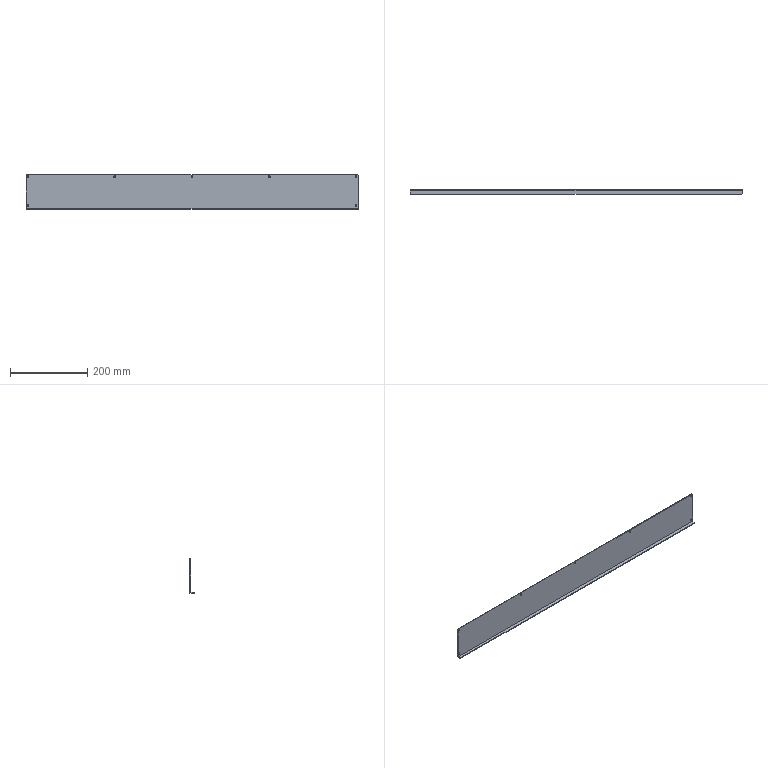Part | NX | 1 solid | 19 faces | box 860 x 10.5 x 89 mm | volume 167461 mm3 | plane 12 | cylinder 7 | commonest cylinder face diameters 4.5 x7
STEP:
#1=CARTESIAN_POINT('',(-430.,0.,-87.));
#2=VERTEX_POINT('',#1);
#3=CARTESIAN_POINT('',(-430.,-6.5,-87.));
#4=VERTEX_POINT('',#3);
#5=CARTESIAN_POINT('',(-430.,0.,-87.));
#6=DIRECTION('',(0.,-1.,0.));
#7=VECTOR('',#6,1000.);
#8=LINE('',#5,#7);
#9=EDGE_CURVE('',#2,#4,#8,.T.);
#10=ORIENTED_EDGE('',*,*,#9,.T.);
#11=CARTESIAN_POINT('',(-428.,-8.5,-87.));
#12=VERTEX_POINT('',#11);
#13=CARTESIAN_POINT('',(-430.,-6.5,-87.));
#14=DIRECTION('',(-0.7071,0.7071,0.));
#15=VECTOR('',#14,1000.);
#16=LINE('',#13,#15);
#17=EDGE_CURVE('',#4,#12,#16,.F.);
#18=ORIENTED_EDGE('',*,*,#17,.T.);
#19=CARTESIAN_POINT('',(428.,-8.5,-87.));
#20=VERTEX_POINT('',#19);
#21=CARTESIAN_POINT('',(430.,-8.5,-87.));
#22=DIRECTION('',(-1.,0.,0.));
#23=VECTOR('',#22,1000.);
#24=LINE('',#21,#23);
#25=EDGE_CURVE('',#20,#12,#24,.T.);
#26=ORIENTED_EDGE('',*,*,#25,.F.);
#27=CARTESIAN_POINT('',(430.,-6.5,-87.));
#28=VERTEX_POINT('',#27);
#29=CARTESIAN_POINT('',(428.,-8.5,-87.));
#30=DIRECTION('',(0.7071,0.7071,0.));
#31=VECTOR('',#30,1000.);
#32=LINE('',#29,#31);
#33=EDGE_CURVE('',#20,#28,#32,.T.);
#34=ORIENTED_EDGE('',*,*,#33,.T.);
#35=CARTESIAN_POINT('',(430.,0.,-87.));
#36=VERTEX_POINT('',#35);
#37=CARTESIAN_POINT('',(430.,0.,-87.));
#38=DIRECTION('',(0.,-1.,0.));
#39=VECTOR('',#38,1000.);
#40=LINE('',#37,#39);
#41=EDGE_CURVE('',#36,#28,#40,.T.);
#42=ORIENTED_EDGE('',*,*,#41,.F.);
#43=CARTESIAN_POINT('',(430.,0.,-87.));
#44=DIRECTION('',(-1.,0.,0.));
#45=VECTOR('',#44,1000.);
#46=LINE('',#43,#45);
#47=EDGE_CURVE('',#36,#2,#46,.T.);
#48=ORIENTED_EDGE('',*,*,#47,.T.);
#49=EDGE_LOOP('',(#10,#18,#26,#34,#42,#48));
#50=FACE_BOUND('',#49,.T.);
#51=CARTESIAN_POINT('',(430.,0.,-87.));
#52=DIRECTION('',(0.,0.,-1.));
#53=DIRECTION('',(-1.,0.,0.));
#54=AXIS2_PLACEMENT_3D('',#51,#52,#53);
#55=PLANE('',#54);
#56=ADVANCED_FACE('',(#50),#55,.F.);
#57=ORIENTED_EDGE('',*,*,#25,.T.);
#58=CARTESIAN_POINT('',(-428.,-8.5,-89.));
#59=VERTEX_POINT('',#58);
#60=CARTESIAN_POINT('',(-428.,-8.5,-89.));
#61=DIRECTION('',(0.,0.,-1.));
#62=VECTOR('',#61,1000.);
#63=LINE('',#60,#62);
#64=EDGE_CURVE('',#12,#59,#63,.T.);
#65=ORIENTED_EDGE('',*,*,#64,.T.);
#66=CARTESIAN_POINT('',(428.,-8.5,-89.));
#67=VERTEX_POINT('',#66);
#68=CARTESIAN_POINT('',(430.,-8.5,-89.));
#69=DIRECTION('',(-1.,0.,0.));
#70=VECTOR('',#69,1000.);
#71=LINE('',#68,#70);
#72=EDGE_CURVE('',#67,#59,#71,.T.);
#73=ORIENTED_EDGE('',*,*,#72,.F.);
#74=CARTESIAN_POINT('',(428.,-8.5,-87.));
#75=DIRECTION('',(0.,0.,1.));
#76=VECTOR('',#75,1000.);
#77=LINE('',#74,#76);
#78=EDGE_CURVE('',#67,#20,#77,.T.);
#79=ORIENTED_EDGE('',*,*,#78,.T.);
#80=EDGE_LOOP('',(#57,#65,#73,#79));
#81=FACE_BOUND('',#80,.T.);
#82=CARTESIAN_POINT('',(430.,-8.5,-89.));
#83=DIRECTION('',(0.,-1.,0.));
#84=DIRECTION('',(0.,0.,-1.));
#85=AXIS2_PLACEMENT_3D('',#82,#83,#84);
#86=PLANE('',#85);
#87=ADVANCED_FACE('',(#81),#86,.T.);
#88=ORIENTED_EDGE('',*,*,#72,.T.);
#89=CARTESIAN_POINT('',(-430.,-6.5,-89.));
#90=VERTEX_POINT('',#89);
#91=CARTESIAN_POINT('',(-3.25,-433.25,-89.));
#92=DIRECTION('',(0.7071,-0.7071,0.));
#93=VECTOR('',#92,1000.);
#94=LINE('',#91,#93);
#95=EDGE_CURVE('',#59,#90,#94,.F.);
#96=ORIENTED_EDGE('',*,*,#95,.T.);
#97=CARTESIAN_POINT('',(-430.,2.,-89.));
#98=VERTEX_POINT('',#97);
#99=CARTESIAN_POINT('',(-430.,0.,-89.));
#100=DIRECTION('',(0.,1.,0.));
#101=VECTOR('',#100,1000.);
#102=LINE('',#99,#101);
#103=EDGE_CURVE('',#98,#90,#102,.F.);
#104=ORIENTED_EDGE('',*,*,#103,.F.);
#105=CARTESIAN_POINT('',(430.,2.,-89.));
#106=VERTEX_POINT('',#105);
#107=CARTESIAN_POINT('',(430.,2.,-89.));
#108=DIRECTION('',(-1.,0.,0.));
#109=VECTOR('',#108,1000.);
#110=LINE('',#107,#109);
#111=EDGE_CURVE('',#106,#98,#110,.T.);
#112=ORIENTED_EDGE('',*,*,#111,.F.);
#113=CARTESIAN_POINT('',(430.,-6.5,-89.));
#114=VERTEX_POINT('',#113);
#115=CARTESIAN_POINT('',(430.,0.,-89.));
#116=DIRECTION('',(0.,1.,0.));
#117=VECTOR('',#116,1000.);
#118=LINE('',#115,#117);
#119=EDGE_CURVE('',#106,#114,#118,.F.);
#120=ORIENTED_EDGE('',*,*,#119,.T.);
#121=CARTESIAN_POINT('',(433.25,-3.25,-89.));
#122=DIRECTION('',(-0.7071,-0.7071,0.));
#123=VECTOR('',#122,1000.);
#124=LINE('',#121,#123);
#125=EDGE_CURVE('',#114,#67,#124,.T.);
#126=ORIENTED_EDGE('',*,*,#125,.T.);
#127=EDGE_LOOP('',(#88,#96,#104,#112,#120,#126));
#128=FACE_BOUND('',#127,.T.);
#129=CARTESIAN_POINT('',(430.,0.,-89.));
#130=DIRECTION('',(0.,0.,-1.));
#131=DIRECTION('',(-1.,0.,0.));
#132=AXIS2_PLACEMENT_3D('',#129,#130,#131);
#133=PLANE('',#132);
#134=ADVANCED_FACE('',(#128),#133,.T.);
#135=CARTESIAN_POINT('',(-425.,2.,-77.75));
#136=VERTEX_POINT('',#135);
#137=CARTESIAN_POINT('',(-425.,2.,-80.));
#138=DIRECTION('',(0.,1.,0.));
#139=DIRECTION('',(0.,0.,1.));
#140=AXIS2_PLACEMENT_3D('',#137,#138,#139);
#141=CIRCLE('',#140,2.25);
#142=EDGE_CURVE('',#136,#136,#141,.T.);
#143=ORIENTED_EDGE('',*,*,#142,.F.);
#144=EDGE_LOOP('',(#143));
#145=FACE_BOUND('',#144,.T.);
#146=CARTESIAN_POINT('',(425.,2.,-77.75));
#147=VERTEX_POINT('',#146);
#148=CARTESIAN_POINT('',(425.,2.,-80.));
#149=DIRECTION('',(0.,1.,0.));
#150=DIRECTION('',(0.,0.,1.));
#151=AXIS2_PLACEMENT_3D('',#148,#149,#150);
#152=CIRCLE('',#151,2.25);
#153=EDGE_CURVE('',#147,#147,#152,.T.);
#154=ORIENTED_EDGE('',*,*,#153,.F.);
#155=EDGE_LOOP('',(#154));
#156=FACE_BOUND('',#155,.T.);
#157=CARTESIAN_POINT('',(-425.,2.,-2.75));
#158=VERTEX_POINT('',#157);
#159=CARTESIAN_POINT('',(-425.,2.,-5.));
#160=DIRECTION('',(0.,1.,0.));
#161=DIRECTION('',(0.,0.,1.));
#162=AXIS2_PLACEMENT_3D('',#159,#160,#161);
#163=CIRCLE('',#162,2.25);
#164=EDGE_CURVE('',#158,#158,#163,.T.);
#165=ORIENTED_EDGE('',*,*,#164,.F.);
#166=EDGE_LOOP('',(#165));
#167=FACE_BOUND('',#166,.T.);
#168=CARTESIAN_POINT('',(425.,2.,-2.75));
#169=VERTEX_POINT('',#168);
#170=CARTESIAN_POINT('',(425.,2.,-5.));
#171=DIRECTION('',(0.,1.,0.));
#172=DIRECTION('',(0.,0.,1.));
#173=AXIS2_PLACEMENT_3D('',#170,#171,#172);
#174=CIRCLE('',#173,2.25);
#175=EDGE_CURVE('',#169,#169,#174,.T.);
#176=ORIENTED_EDGE('',*,*,#175,.F.);
#177=EDGE_LOOP('',(#176));
#178=FACE_BOUND('',#177,.T.);
#179=CARTESIAN_POINT('',(200.,2.,-2.75));
#180=VERTEX_POINT('',#179);
#181=CARTESIAN_POINT('',(200.,2.,-5.));
#182=DIRECTION('',(0.,1.,0.));
#183=DIRECTION('',(0.,0.,1.));
#184=AXIS2_PLACEMENT_3D('',#181,#182,#183);
#185=CIRCLE('',#184,2.25);
#186=EDGE_CURVE('',#180,#180,#185,.T.);
#187=ORIENTED_EDGE('',*,*,#186,.F.);
#188=EDGE_LOOP('',(#187));
#189=FACE_BOUND('',#188,.T.);
#190=CARTESIAN_POINT('',(-200.,2.,-2.75));
#191=VERTEX_POINT('',#190);
#192=CARTESIAN_POINT('',(-200.,2.,-5.));
#193=DIRECTION('',(0.,1.,0.));
#194=DIRECTION('',(0.,0.,1.));
#195=AXIS2_PLACEMENT_3D('',#192,#193,#194);
#196=CIRCLE('',#195,2.25);
#197=EDGE_CURVE('',#191,#191,#196,.T.);
#198=ORIENTED_EDGE('',*,*,#197,.F.);
#199=EDGE_LOOP('',(#198));
#200=FACE_BOUND('',#199,.T.);
#201=CARTESIAN_POINT('',(0.,2.,-2.75));
#202=VERTEX_POINT('',#201);
#203=CARTESIAN_POINT('',(0.,2.,-5.));
#204=DIRECTION('',(0.,1.,0.));
#205=DIRECTION('',(0.,0.,1.));
#206=AXIS2_PLACEMENT_3D('',#203,#204,#205);
#207=CIRCLE('',#206,2.25);
#208=EDGE_CURVE('',#202,#202,#207,.T.);
#209=ORIENTED_EDGE('',*,*,#208,.F.);
#210=EDGE_LOOP('',(#209));
#211=FACE_BOUND('',#210,.T.);
#212=CARTESIAN_POINT('',(428.,2.,0.));
#213=VERTEX_POINT('',#212);
#214=CARTESIAN_POINT('',(-428.,2.,0.));
#215=VERTEX_POINT('',#214);
#216=CARTESIAN_POINT('',(430.,2.,0.));
#217=DIRECTION('',(-1.,0.,0.));
#218=VECTOR('',#217,1000.);
#219=LINE('',#216,#218);
#220=EDGE_CURVE('',#213,#215,#219,.T.);
#221=ORIENTED_EDGE('',*,*,#220,.F.);
#222=CARTESIAN_POINT('',(430.,2.,-2.));
#223=VERTEX_POINT('',#222);
#224=CARTESIAN_POINT('',(429.,2.,-1.));
#225=DIRECTION('',(0.7071,0.,-0.7071));
#226=VECTOR('',#225,1000.);
#227=LINE('',#224,#226);
#228=EDGE_CURVE('',#213,#223,#227,.T.);
#229=ORIENTED_EDGE('',*,*,#228,.T.);
#230=CARTESIAN_POINT('',(430.,2.,0.));
#231=DIRECTION('',(0.,0.,-1.));
#232=VECTOR('',#231,1000.);
#233=LINE('',#230,#232);
#234=EDGE_CURVE('',#223,#106,#233,.T.);
#235=ORIENTED_EDGE('',*,*,#234,.T.);
#236=ORIENTED_EDGE('',*,*,#111,.T.);
#237=CARTESIAN_POINT('',(-430.,2.,-2.));
#238=VERTEX_POINT('',#237);
#239=CARTESIAN_POINT('',(-430.,2.,0.));
#240=DIRECTION('',(0.,0.,-1.));
#241=VECTOR('',#240,1000.);
#242=LINE('',#239,#241);
#243=EDGE_CURVE('',#238,#98,#242,.T.);
#244=ORIENTED_EDGE('',*,*,#243,.F.);
#245=CARTESIAN_POINT('',(1.,2.,429.));
#246=DIRECTION('',(-0.7071,0.,-0.7071));
#247=VECTOR('',#246,1000.);
#248=LINE('',#245,#247);
#249=EDGE_CURVE('',#238,#215,#248,.F.);
#250=ORIENTED_EDGE('',*,*,#249,.T.);
#251=EDGE_LOOP('',(#221,#229,#235,#236,#244,#250));
#252=FACE_BOUND('',#251,.T.);
#253=CARTESIAN_POINT('',(430.,2.,0.));
#254=DIRECTION('',(0.,1.,0.));
#255=DIRECTION('',(0.,0.,1.));
#256=AXIS2_PLACEMENT_3D('',#253,#254,#255);
#257=PLANE('',#256);
#258=ADVANCED_FACE('',(#145,#156,#167,#178,#189,#200,#211,#252),#257,.T.);
#259=CARTESIAN_POINT('',(428.,0.,0.));
#260=VERTEX_POINT('',#259);
#261=CARTESIAN_POINT('',(-428.,0.,0.));
#262=VERTEX_POINT('',#261);
#263=CARTESIAN_POINT('',(430.,0.,0.));
#264=DIRECTION('',(-1.,0.,0.));
#265=VECTOR('',#264,1000.);
#266=LINE('',#263,#265);
#267=EDGE_CURVE('',#260,#262,#266,.T.);
#268=ORIENTED_EDGE('',*,*,#267,.F.);
#269=CARTESIAN_POINT('',(428.,2.,0.));
#270=DIRECTION('',(0.,1.,0.));
#271=VECTOR('',#270,1000.);
#272=LINE('',#269,#271);
#273=EDGE_CURVE('',#260,#213,#272,.T.);
#274=ORIENTED_EDGE('',*,*,#273,.T.);
#275=ORIENTED_EDGE('',*,*,#220,.T.);
#276=CARTESIAN_POINT('',(-428.,0.,0.));
#277=DIRECTION('',(0.,-1.,0.));
#278=VECTOR('',#277,1000.);
#279=LINE('',#276,#278);
#280=EDGE_CURVE('',#215,#262,#279,.T.);
#281=ORIENTED_EDGE('',*,*,#280,.T.);
#282=EDGE_LOOP('',(#268,#274,#275,#281));
#283=FACE_BOUND('',#282,.T.);
#284=CARTESIAN_POINT('',(430.,0.,0.));
#285=DIRECTION('',(0.,0.,1.));
#286=DIRECTION('',(1.,0.,0.));
#287=AXIS2_PLACEMENT_3D('',#284,#285,#286);
#288=PLANE('',#287);
#289=ADVANCED_FACE('',(#283),#288,.T.);
#290=CARTESIAN_POINT('',(-425.,0.,-77.75));
#291=VERTEX_POINT('',#290);
#292=CARTESIAN_POINT('',(-425.,0.,-80.));
#293=DIRECTION('',(0.,1.,0.));
#294=DIRECTION('',(0.,0.,1.));
#295=AXIS2_PLACEMENT_3D('',#292,#293,#294);
#296=CIRCLE('',#295,2.25);
#297=EDGE_CURVE('',#291,#291,#296,.T.);
#298=ORIENTED_EDGE('',*,*,#297,.T.);
#299=EDGE_LOOP('',(#298));
#300=FACE_BOUND('',#299,.T.);
#301=CARTESIAN_POINT('',(425.,0.,-77.75));
#302=VERTEX_POINT('',#301);
#303=CARTESIAN_POINT('',(425.,0.,-80.));
#304=DIRECTION('',(0.,1.,0.));
#305=DIRECTION('',(0.,0.,1.));
#306=AXIS2_PLACEMENT_3D('',#303,#304,#305);
#307=CIRCLE('',#306,2.25);
#308=EDGE_CURVE('',#302,#302,#307,.T.);
#309=ORIENTED_EDGE('',*,*,#308,.T.);
#310=EDGE_LOOP('',(#309));
#311=FACE_BOUND('',#310,.T.);
#312=CARTESIAN_POINT('',(-425.,0.,-2.75));
#313=VERTEX_POINT('',#312);
#314=CARTESIAN_POINT('',(-425.,0.,-5.));
#315=DIRECTION('',(0.,1.,0.));
#316=DIRECTION('',(0.,0.,1.));
#317=AXIS2_PLACEMENT_3D('',#314,#315,#316);
#318=CIRCLE('',#317,2.25);
#319=EDGE_CURVE('',#313,#313,#318,.T.);
#320=ORIENTED_EDGE('',*,*,#319,.T.);
#321=EDGE_LOOP('',(#320));
#322=FACE_BOUND('',#321,.T.);
#323=CARTESIAN_POINT('',(425.,0.,-2.75));
#324=VERTEX_POINT('',#323);
#325=CARTESIAN_POINT('',(425.,0.,-5.));
#326=DIRECTION('',(0.,1.,0.));
#327=DIRECTION('',(0.,0.,1.));
#328=AXIS2_PLACEMENT_3D('',#325,#326,#327);
#329=CIRCLE('',#328,2.25);
#330=EDGE_CURVE('',#324,#324,#329,.T.);
#331=ORIENTED_EDGE('',*,*,#330,.T.);
#332=EDGE_LOOP('',(#331));
#333=FACE_BOUND('',#332,.T.);
#334=CARTESIAN_POINT('',(200.,0.,-2.75));
#335=VERTEX_POINT('',#334);
#336=CARTESIAN_POINT('',(200.,0.,-5.));
#337=DIRECTION('',(0.,1.,0.));
#338=DIRECTION('',(0.,0.,1.));
#339=AXIS2_PLACEMENT_3D('',#336,#337,#338);
#340=CIRCLE('',#339,2.25);
#341=EDGE_CURVE('',#335,#335,#340,.T.);
#342=ORIENTED_EDGE('',*,*,#341,.T.);
#343=EDGE_LOOP('',(#342));
#344=FACE_BOUND('',#343,.T.);
#345=CARTESIAN_POINT('',(-200.,0.,-2.75));
#346=VERTEX_POINT('',#345);
#347=CARTESIAN_POINT('',(-200.,0.,-5.));
#348=DIRECTION('',(0.,1.,0.));
#349=DIRECTION('',(0.,0.,1.));
#350=AXIS2_PLACEMENT_3D('',#347,#348,#349);
#351=CIRCLE('',#350,2.25);
#352=EDGE_CURVE('',#346,#346,#351,.T.);
#353=ORIENTED_EDGE('',*,*,#352,.T.);
#354=EDGE_LOOP('',(#353));
#355=FACE_BOUND('',#354,.T.);
#356=CARTESIAN_POINT('',(0.,0.,-2.75));
#357=VERTEX_POINT('',#356);
#358=CARTESIAN_POINT('',(0.,0.,-5.));
#359=DIRECTION('',(0.,1.,0.));
#360=DIRECTION('',(0.,0.,1.));
#361=AXIS2_PLACEMENT_3D('',#358,#359,#360);
#362=CIRCLE('',#361,2.25);
#363=EDGE_CURVE('',#357,#357,#362,.T.);
#364=ORIENTED_EDGE('',*,*,#363,.T.);
#365=EDGE_LOOP('',(#364));
#366=FACE_BOUND('',#365,.T.);
#367=CARTESIAN_POINT('',(430.,0.,-2.));
#368=VERTEX_POINT('',#367);
#369=CARTESIAN_POINT('',(430.,0.,0.));
#370=DIRECTION('',(0.,0.,-1.));
#371=VECTOR('',#370,1000.);
#372=LINE('',#369,#371);
#373=EDGE_CURVE('',#368,#36,#372,.T.);
#374=ORIENTED_EDGE('',*,*,#373,.F.);
#375=CARTESIAN_POINT('',(428.,0.,0.));
#376=DIRECTION('',(-0.7071,0.,0.7071));
#377=VECTOR('',#376,1000.);
#378=LINE('',#375,#377);
#379=EDGE_CURVE('',#368,#260,#378,.T.);
#380=ORIENTED_EDGE('',*,*,#379,.T.);
#381=ORIENTED_EDGE('',*,*,#267,.T.);
#382=CARTESIAN_POINT('',(-430.,0.,-2.));
#383=VERTEX_POINT('',#382);
#384=CARTESIAN_POINT('',(-430.,0.,-2.));
#385=DIRECTION('',(0.7071,0.,0.7071));
#386=VECTOR('',#385,1000.);
#387=LINE('',#384,#386);
#388=EDGE_CURVE('',#262,#383,#387,.F.);
#389=ORIENTED_EDGE('',*,*,#388,.T.);
#390=CARTESIAN_POINT('',(-430.,0.,0.));
#391=DIRECTION('',(0.,0.,-1.));
#392=VECTOR('',#391,1000.);
#393=LINE('',#390,#392);
#394=EDGE_CURVE('',#383,#2,#393,.T.);
#395=ORIENTED_EDGE('',*,*,#394,.T.);
#396=ORIENTED_EDGE('',*,*,#47,.F.);
#397=EDGE_LOOP('',(#374,#380,#381,#389,#395,#396));
#398=FACE_BOUND('',#397,.T.);
#399=CARTESIAN_POINT('',(430.,0.,0.));
#400=DIRECTION('',(0.,1.,0.));
#401=DIRECTION('',(0.,0.,1.));
#402=AXIS2_PLACEMENT_3D('',#399,#400,#401);
#403=PLANE('',#402);
#404=ADVANCED_FACE('',(#300,#311,#322,#333,#344,#355,#366,#398),#403,.F.);
#405=ORIENTED_EDGE('',*,*,#234,.F.);
#406=CARTESIAN_POINT('',(430.,0.,-2.));
#407=DIRECTION('',(0.,-1.,0.));
#408=VECTOR('',#407,1000.);
#409=LINE('',#406,#408);
#410=EDGE_CURVE('',#223,#368,#409,.T.);
#411=ORIENTED_EDGE('',*,*,#410,.T.);
#412=ORIENTED_EDGE('',*,*,#373,.T.);
#413=ORIENTED_EDGE('',*,*,#41,.T.);
#414=CARTESIAN_POINT('',(430.,-6.5,-89.));
#415=DIRECTION('',(0.,0.,-1.));
#416=VECTOR('',#415,1000.);
#417=LINE('',#414,#416);
#418=EDGE_CURVE('',#28,#114,#417,.T.);
#419=ORIENTED_EDGE('',*,*,#418,.T.);
#420=ORIENTED_EDGE('',*,*,#119,.F.);
#421=EDGE_LOOP('',(#405,#411,#412,#413,#419,#420));
#422=FACE_BOUND('',#421,.T.);
#423=CARTESIAN_POINT('',(430.,0.,0.));
#424=DIRECTION('',(-1.,0.,0.));
#425=DIRECTION('',(0.,0.,1.));
#426=AXIS2_PLACEMENT_3D('',#423,#424,#425);
#427=PLANE('',#426);
#428=ADVANCED_FACE('',(#422),#427,.F.);
#429=ORIENTED_EDGE('',*,*,#394,.F.);
#430=CARTESIAN_POINT('',(-430.,0.,-2.));
#431=DIRECTION('',(0.,1.,0.));
#432=VECTOR('',#431,1000.);
#433=LINE('',#430,#432);
#434=EDGE_CURVE('',#383,#238,#433,.T.);
#435=ORIENTED_EDGE('',*,*,#434,.T.);
#436=ORIENTED_EDGE('',*,*,#243,.T.);
#437=ORIENTED_EDGE('',*,*,#103,.T.);
#438=CARTESIAN_POINT('',(-430.,-6.5,0.));
#439=DIRECTION('',(0.,0.,1.));
#440=VECTOR('',#439,1000.);
#441=LINE('',#438,#440);
#442=EDGE_CURVE('',#90,#4,#441,.T.);
#443=ORIENTED_EDGE('',*,*,#442,.T.);
#444=ORIENTED_EDGE('',*,*,#9,.F.);
#445=EDGE_LOOP('',(#429,#435,#436,#437,#443,#444));
#446=FACE_BOUND('',#445,.T.);
#447=CARTESIAN_POINT('',(-430.,0.,0.));
#448=DIRECTION('',(-1.,0.,0.));
#449=DIRECTION('',(0.,0.,1.));
#450=AXIS2_PLACEMENT_3D('',#447,#448,#449);
#451=PLANE('',#450);
#452=ADVANCED_FACE('',(#446),#451,.T.);
#453=ORIENTED_EDGE('',*,*,#379,.F.);
#454=ORIENTED_EDGE('',*,*,#410,.F.);
#455=ORIENTED_EDGE('',*,*,#228,.F.);
#456=ORIENTED_EDGE('',*,*,#273,.F.);
#457=EDGE_LOOP('',(#453,#454,#455,#456));
#458=FACE_BOUND('',#457,.T.);
#459=CARTESIAN_POINT('',(428.,0.,0.));
#460=DIRECTION('',(0.7071,0.,0.7071));
#461=DIRECTION('',(0.,-1.,0.));
#462=AXIS2_PLACEMENT_3D('',#459,#460,#461);
#463=PLANE('',#462);
#464=ADVANCED_FACE('',(#458),#463,.T.);
#465=ORIENTED_EDGE('',*,*,#388,.F.);
#466=ORIENTED_EDGE('',*,*,#280,.F.);
#467=ORIENTED_EDGE('',*,*,#249,.F.);
#468=ORIENTED_EDGE('',*,*,#434,.F.);
#469=EDGE_LOOP('',(#465,#466,#467,#468));
#470=FACE_BOUND('',#469,.T.);
#471=CARTESIAN_POINT('',(-430.,0.,-2.));
#472=DIRECTION('',(0.7071,0.,-0.7071));
#473=DIRECTION('',(0.,1.,0.));
#474=AXIS2_PLACEMENT_3D('',#471,#472,#473);
#475=PLANE('',#474);
#476=ADVANCED_FACE('',(#470),#475,.F.);
#477=ORIENTED_EDGE('',*,*,#95,.F.);
#478=ORIENTED_EDGE('',*,*,#64,.F.);
#479=ORIENTED_EDGE('',*,*,#17,.F.);
#480=ORIENTED_EDGE('',*,*,#442,.F.);
#481=EDGE_LOOP('',(#477,#478,#479,#480));
#482=FACE_BOUND('',#481,.T.);
#483=CARTESIAN_POINT('',(-430.,-6.5,0.));
#484=DIRECTION('',(0.7071,0.7071,0.));
#485=DIRECTION('',(0.,0.,1.));
#486=AXIS2_PLACEMENT_3D('',#483,#484,#485);
#487=PLANE('',#486);
#488=ADVANCED_FACE('',(#482),#487,.F.);
#489=ORIENTED_EDGE('',*,*,#125,.F.);
#490=ORIENTED_EDGE('',*,*,#418,.F.);
#491=ORIENTED_EDGE('',*,*,#33,.F.);
#492=ORIENTED_EDGE('',*,*,#78,.F.);
#493=EDGE_LOOP('',(#489,#490,#491,#492));
#494=FACE_BOUND('',#493,.T.);
#495=CARTESIAN_POINT('',(428.,-8.5,-89.));
#496=DIRECTION('',(0.7071,-0.7071,0.));
#497=DIRECTION('',(0.,0.,-1.));
#498=AXIS2_PLACEMENT_3D('',#495,#496,#497);
#499=PLANE('',#498);
#500=ADVANCED_FACE('',(#494),#499,.T.);
#501=ORIENTED_EDGE('',*,*,#208,.T.);
#502=EDGE_LOOP('',(#501));
#503=FACE_BOUND('',#502,.T.);
#504=ORIENTED_EDGE('',*,*,#363,.F.);
#505=EDGE_LOOP('',(#504));
#506=FACE_BOUND('',#505,.T.);
#507=CARTESIAN_POINT('',(0.,2.,-5.));
#508=DIRECTION('',(0.,1.,0.));
#509=DIRECTION('',(0.,0.,1.));
#510=AXIS2_PLACEMENT_3D('',#507,#508,#509);
#511=CYLINDRICAL_SURFACE('',#510,2.25);
#512=ADVANCED_FACE('',(#503,#506),#511,.F.);
#513=ORIENTED_EDGE('',*,*,#197,.T.);
#514=EDGE_LOOP('',(#513));
#515=FACE_BOUND('',#514,.T.);
#516=ORIENTED_EDGE('',*,*,#352,.F.);
#517=EDGE_LOOP('',(#516));
#518=FACE_BOUND('',#517,.T.);
#519=CARTESIAN_POINT('',(-200.,2.,-5.));
#520=DIRECTION('',(0.,1.,0.));
#521=DIRECTION('',(0.,0.,1.));
#522=AXIS2_PLACEMENT_3D('',#519,#520,#521);
#523=CYLINDRICAL_SURFACE('',#522,2.25);
#524=ADVANCED_FACE('',(#515,#518),#523,.F.);
#525=ORIENTED_EDGE('',*,*,#186,.T.);
#526=EDGE_LOOP('',(#525));
#527=FACE_BOUND('',#526,.T.);
#528=ORIENTED_EDGE('',*,*,#341,.F.);
#529=EDGE_LOOP('',(#528));
#530=FACE_BOUND('',#529,.T.);
#531=CARTESIAN_POINT('',(200.,2.,-5.));
#532=DIRECTION('',(0.,1.,0.));
#533=DIRECTION('',(0.,0.,1.));
#534=AXIS2_PLACEMENT_3D('',#531,#532,#533);
#535=CYLINDRICAL_SURFACE('',#534,2.25);
#536=ADVANCED_FACE('',(#527,#530),#535,.F.);
#537=ORIENTED_EDGE('',*,*,#175,.T.);
#538=EDGE_LOOP('',(#537));
#539=FACE_BOUND('',#538,.T.);
#540=ORIENTED_EDGE('',*,*,#330,.F.);
#541=EDGE_LOOP('',(#540));
#542=FACE_BOUND('',#541,.T.);
#543=CARTESIAN_POINT('',(425.,2.,-5.));
#544=DIRECTION('',(0.,1.,0.));
#545=DIRECTION('',(0.,0.,1.));
#546=AXIS2_PLACEMENT_3D('',#543,#544,#545);
#547=CYLINDRICAL_SURFACE('',#546,2.25);
#548=ADVANCED_FACE('',(#539,#542),#547,.F.);
#549=ORIENTED_EDGE('',*,*,#164,.T.);
#550=EDGE_LOOP('',(#549));
#551=FACE_BOUND('',#550,.T.);
#552=ORIENTED_EDGE('',*,*,#319,.F.);
#553=EDGE_LOOP('',(#552));
#554=FACE_BOUND('',#553,.T.);
#555=CARTESIAN_POINT('',(-425.,2.,-5.));
#556=DIRECTION('',(0.,1.,0.));
#557=DIRECTION('',(0.,0.,1.));
#558=AXIS2_PLACEMENT_3D('',#555,#556,#557);
#559=CYLINDRICAL_SURFACE('',#558,2.25);
#560=ADVANCED_FACE('',(#551,#554),#559,.F.);
#561=ORIENTED_EDGE('',*,*,#153,.T.);
#562=EDGE_LOOP('',(#561));
#563=FACE_BOUND('',#562,.T.);
#564=ORIENTED_EDGE('',*,*,#308,.F.);
#565=EDGE_LOOP('',(#564));
#566=FACE_BOUND('',#565,.T.);
#567=CARTESIAN_POINT('',(425.,2.,-80.));
#568=DIRECTION('',(0.,1.,0.));
#569=DIRECTION('',(0.,0.,1.));
#570=AXIS2_PLACEMENT_3D('',#567,#568,#569);
#571=CYLINDRICAL_SURFACE('',#570,2.25);
#572=ADVANCED_FACE('',(#563,#566),#571,.F.);
#573=ORIENTED_EDGE('',*,*,#142,.T.);
#574=EDGE_LOOP('',(#573));
#575=FACE_BOUND('',#574,.T.);
#576=ORIENTED_EDGE('',*,*,#297,.F.);
#577=EDGE_LOOP('',(#576));
#578=FACE_BOUND('',#577,.T.);
#579=CARTESIAN_POINT('',(-425.,2.,-80.));
#580=DIRECTION('',(0.,1.,0.));
#581=DIRECTION('',(0.,0.,1.));
#582=AXIS2_PLACEMENT_3D('',#579,#580,#581);
#583=CYLINDRICAL_SURFACE('',#582,2.25);
#584=ADVANCED_FACE('',(#575,#578),#583,.F.);
#585=CLOSED_SHELL('',(#56,#87,#134,#258,#289,#404,#428,#452,#464,#476,#488,#500,#512,#524,#536,#548,#560,#572,#584));
#586=MANIFOLD_SOLID_BREP('',#585);
#587=(LENGTH_UNIT()NAMED_UNIT(*)SI_UNIT(.MILLI.,.METRE.));
#588=UNCERTAINTY_MEASURE_WITH_UNIT(LENGTH_MEASURE(0.00001),#587,'','');
#589=(NAMED_UNIT(*)PLANE_ANGLE_UNIT()SI_UNIT($,.RADIAN.));
#590=(NAMED_UNIT(*)SI_UNIT($,.STERADIAN.)SOLID_ANGLE_UNIT());
#591=(GEOMETRIC_REPRESENTATION_CONTEXT(3)GLOBAL_UNCERTAINTY_ASSIGNED_CONTEXT((#588))GLOBAL_UNIT_ASSIGNED_CONTEXT((#587,#589,#590))REPRESENTATION_CONTEXT('',''));
#592=ADVANCED_BREP_SHAPE_REPRESENTATION('',(#586),#591);